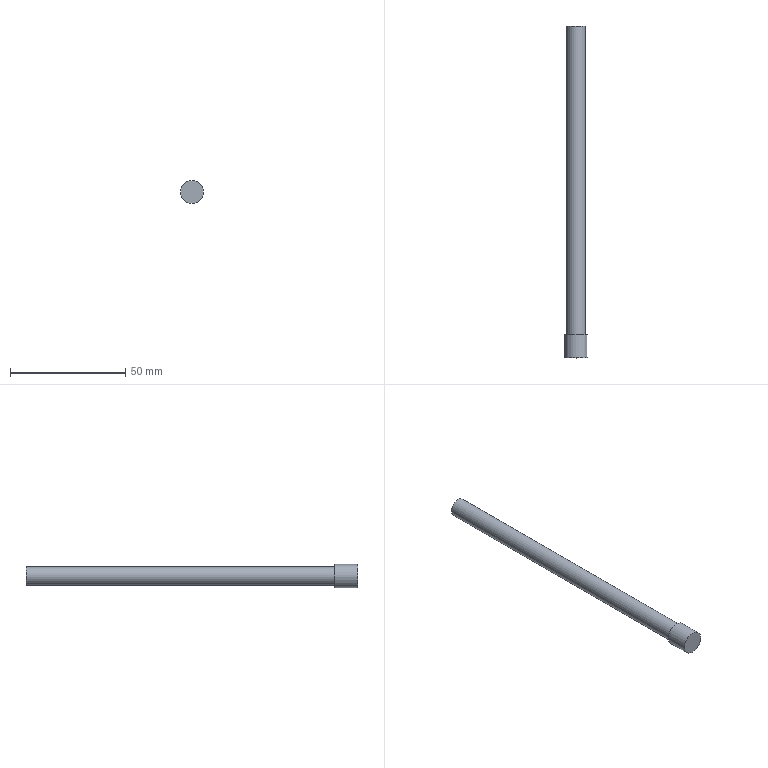Part | STEP file | solid 139 | 1 solid | 5 faces | box 10 x 144 x 10 mm | volume 7521 mm3 | plane 3 | cylinder 2 | commonest cylinder face diameters 8 x1 10 x1